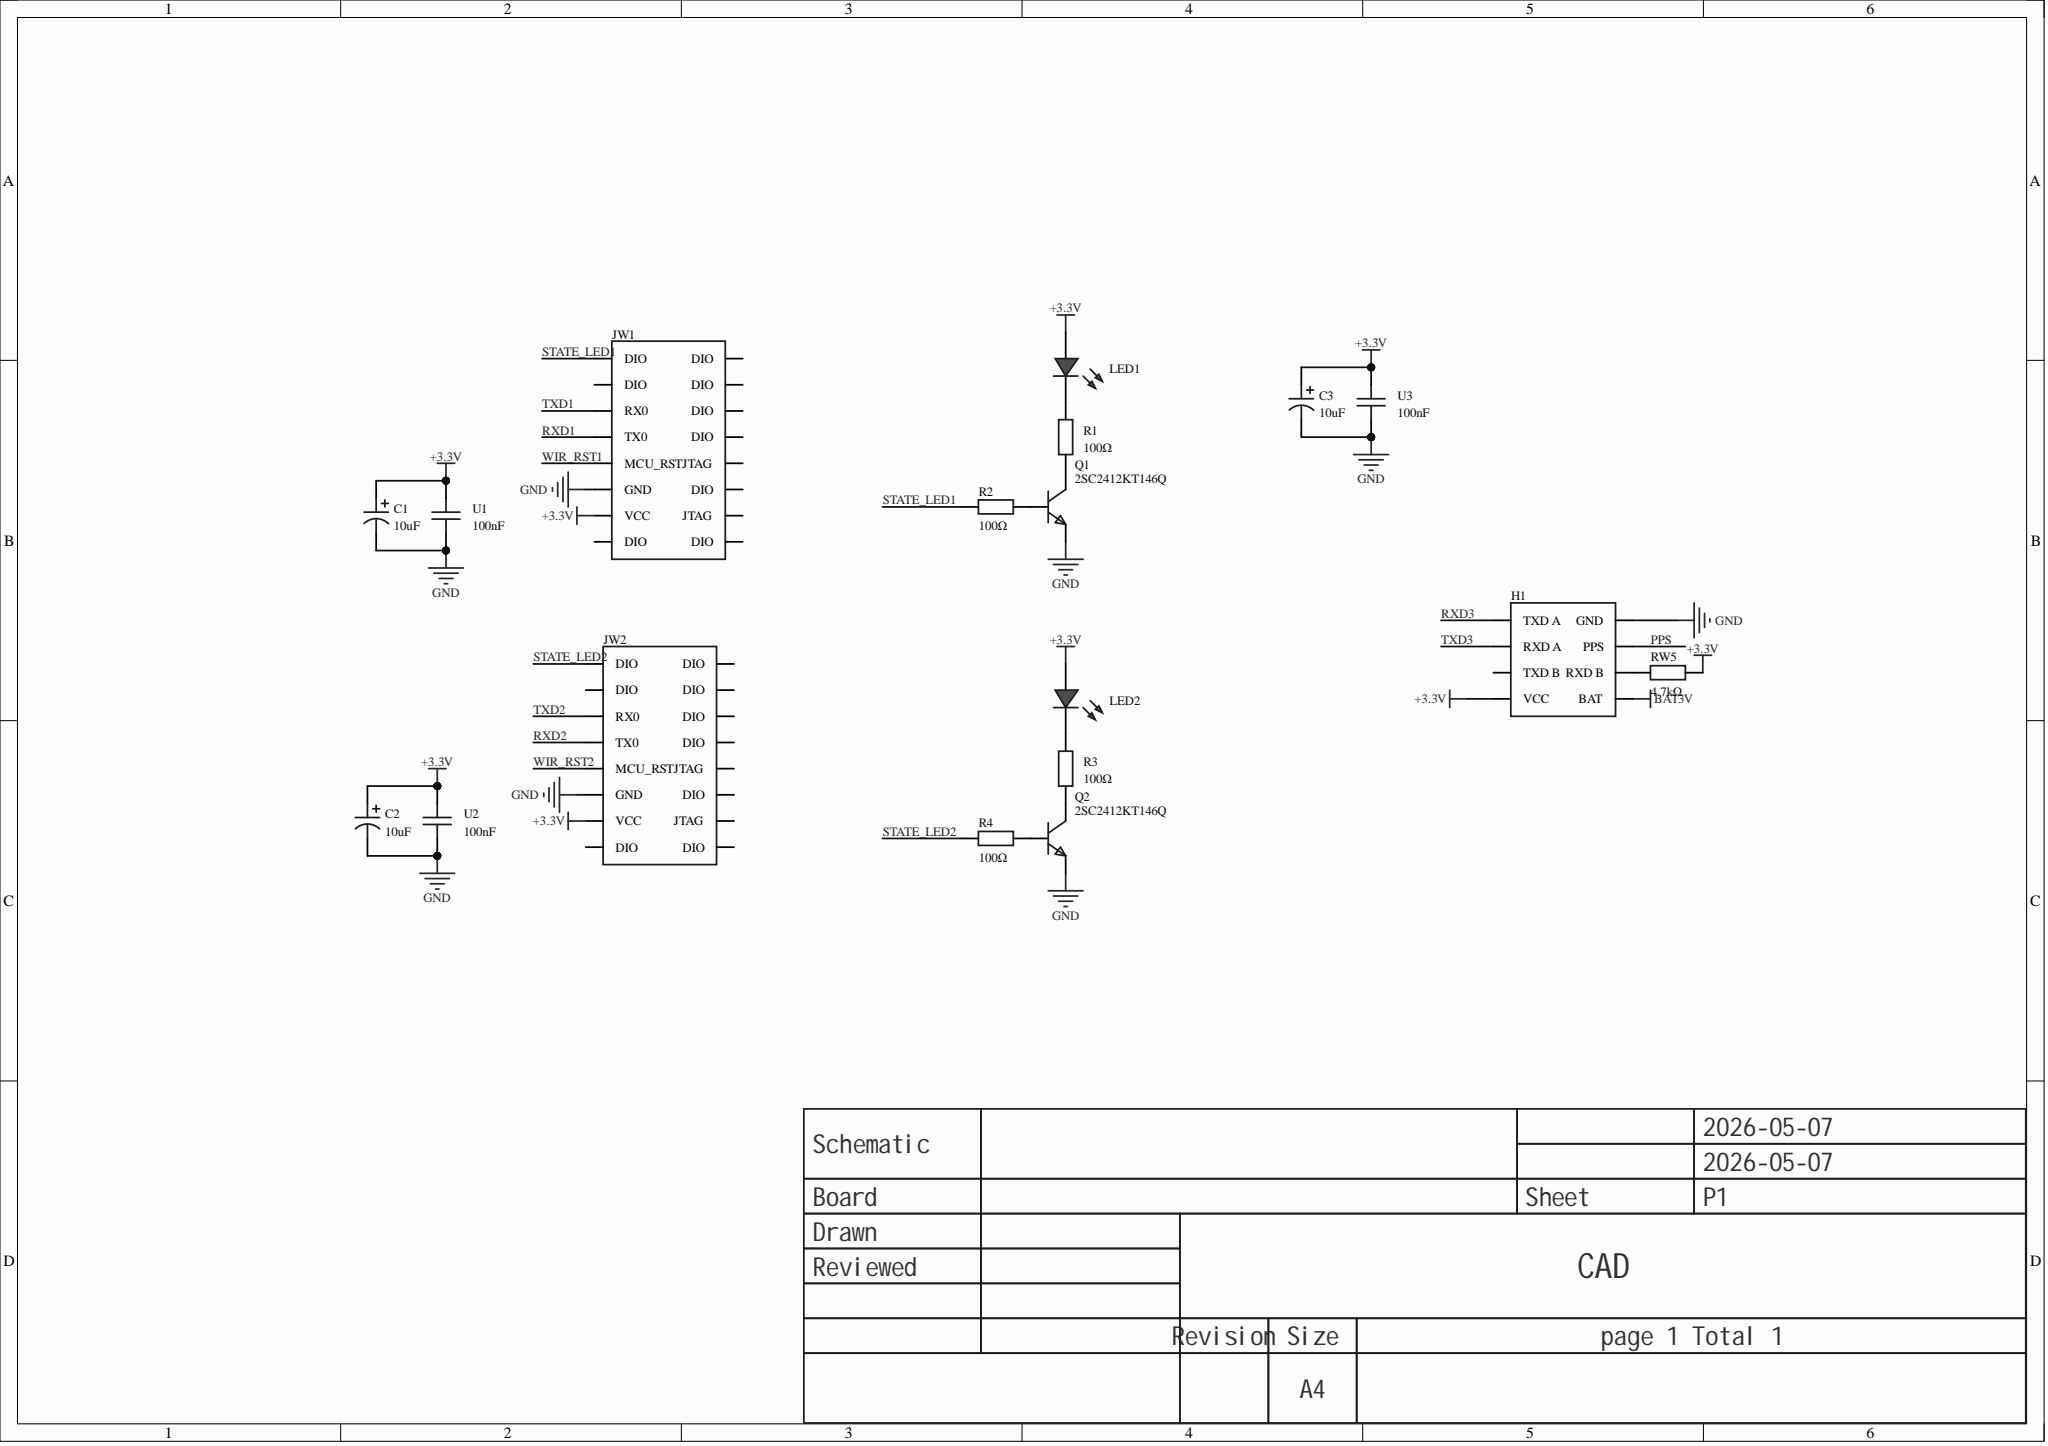Circuit board | Altium Designer | 18 parts | 11 nets
Bill of materials:
Comment,Description,Designator,Footprint,LibRef,Quantity
"10uF","component 10UF50VC110GL componentdescrip capacitance:10uF; tolerance:±20%; rated voltage:50V; ripple current:120mA@100KHz; equivalent series resistance(ESR):1.6Ω;","C1, C2, C3","CAP-TH_BD5.0-P2.00-D0.8-FD-10UF50VC110GL","10UF50VC110GL","3"
"","","H1","HDR-TH_8P-P2.54-V-F-R2-C4-S2.54-1","HDR-F_2.54_2x4","1"
"","","JW1, JW2","HDR-TH_16P-P2.54-V-F-R2-C8-S2.54-1","HDR-F_2.54_2x8","2"
"","","LED1, LED2","LED_TH-3mm","LED_TH-R_3mm","2"
"2SC2412KT146Q","component 2SC2412KT146Q componentdescrip transistor type:NPN; collector current(Ic):150mA; collector-emitter breakdown voltage(Vceo):50V; power dissipation(Pd):200mW; DC current gain(hFE):120@1mA,6V;","Q1, Q2","SOT-346_L2.9-W1.6-P1.90-LS2.8-TR-CW-1","2SC2412KT146Q","2"
"100Ω","","R1, R2, R3, R4","Res_1/8W","Res_AXIAL-1/8W","4"
"4.7kΩ","","RW5","Res_1/8W","Res_AXIAL-1/8W","1"
"100nF","","U1, U2, U3","CAP-TH_L5.0-W2.5-P5.00-D1.0","100nF","3"
Netlist (Protel format):
[
C1
CAP-TH_BD5.0-P2.00-D0.8-FD-10UF50VC110GL
10uF



]
[
C2
CAP-TH_BD5.0-P2.00-D0.8-FD-10UF50VC110GL
10uF



]
[
C3
CAP-TH_BD5.0-P2.00-D0.8-FD-10UF50VC110GL
10uF



]
[
H1
HDR-TH_8P-P2.54-V-F-R2-C4-S2.54-1




]
[
JW1
HDR-TH_16P-P2.54-V-F-R2-C8-S2.54-1




]
[
JW2
HDR-TH_16P-P2.54-V-F-R2-C8-S2.54-1




]
[
LED1
LED_TH-3mm




]
[
LED2
LED_TH-3mm




]
[
Q1
SOT-346_L2.9-W1.6-P1.90-LS2.8-TR-CW-1
2SC2412KT146Q



]
[
Q2
SOT-346_L2.9-W1.6-P1.90-LS2.8-TR-CW-1
2SC2412KT146Q



]
[
R1
Res_1/8W
100Ω



]
[
R2
Res_1/8W
100Ω



]
[
R3
Res_1/8W
100Ω



]
[
R4
Res_1/8W
100Ω



]
[
RW5
Res_1/8W
4.7kΩ



]
[
U1
CAP-TH_L5.0-W2.5-P5.00-D1.0
100nF



]
[
U2
CAP-TH_L5.0-W2.5-P5.00-D1.0
100nF



]
[
U3
CAP-TH_L5.0-W2.5-P5.00-D1.0
100nF



]
(
STATE_LED2
JW2-1
R4-2
)
(
STATE_LED1
JW1-1
R2-2
)
(
NetQ2_3
Q2-3
R3-1
)
(
NetQ2_2
Q2-2
R4-1
)
(
NetQ1_3
Q1-3
R1-1
)
(
NetQ1_2
Q1-2
R2-1
)
(
NetLED2_2
LED2-2
R3-2
)
(
NetLED1_2
LED1-2
R1-2
)
(
NetH1_6
H1-6
RW5-1
)
(
GND
C1-2
C2-2
C3-2
H1-2
JW1-11
JW2-11
Q1-1
Q2-1
U1-2
U2-2
U3-2
)
(
+3.3V
C1-1
C2-1
C3-1
H1-7
JW1-13
JW2-13
LED1-1
LED2-1
RW5-2
U1-1
U2-1
U3-1
)